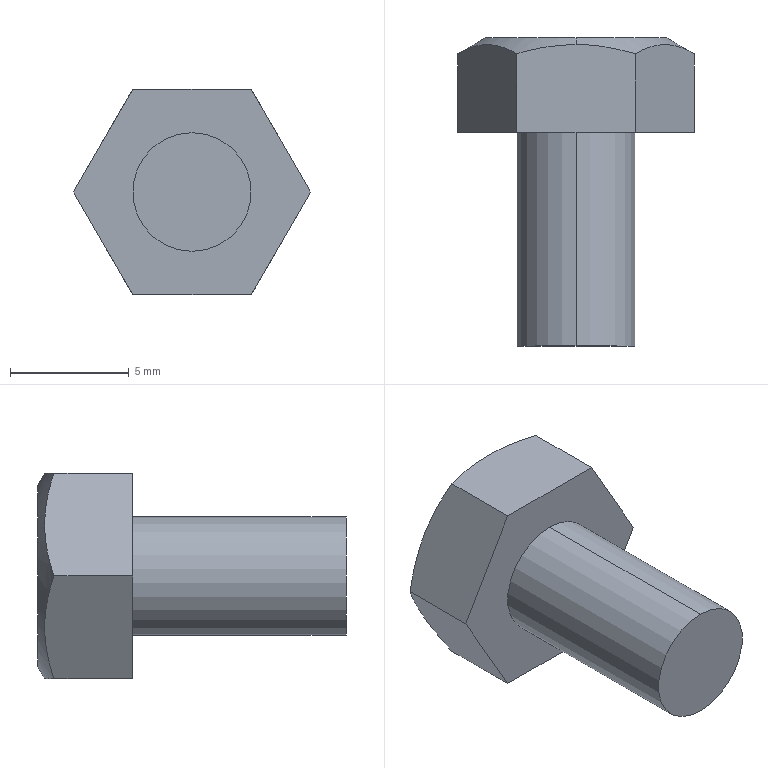Part | SolidWorks | features ICE 2, Extrusion 1 | 1 solid | 13 faces | box 10 x 13 x 8.66 mm | volume 432.272 mm3 | plane 9 | cylinder 2 | cone 2 | commonest cylinder face diameters 5 x2
STEP:
#1=CARTESIAN_POINT('',(0.,-0.3543,-0.09843));
#2=VERTEX_POINT('',#1);
#3=CARTESIAN_POINT('',(0.,-0.3543,0.09843));
#4=VERTEX_POINT('',#3);
#5=CARTESIAN_POINT('',(0.,-0.3543,0.));
#6=DIRECTION('',(0.,-1.,0.));
#7=DIRECTION('',(0.,0.,-1.));
#8=AXIS2_PLACEMENT_3D('',#5,#6,#7);
#9=CIRCLE('',#8,0.09843);
#10=EDGE_CURVE('',#2,#4,#9,.T.);
#11=ORIENTED_EDGE('',*,*,#10,.F.);
#12=CARTESIAN_POINT('',(0.,0.,-0.09843));
#13=VERTEX_POINT('',#12);
#14=CARTESIAN_POINT('',(0.,-0.3543,-0.09843));
#15=DIRECTION('',(0.,1.,0.));
#16=VECTOR('',#15,39.37);
#17=LINE('',#14,#16);
#18=EDGE_CURVE('',#2,#13,#17,.T.);
#19=ORIENTED_EDGE('',*,*,#18,.T.);
#20=CARTESIAN_POINT('',(0.,0.,0.09843));
#21=VERTEX_POINT('',#20);
#22=CARTESIAN_POINT('',(0.,0.,0.));
#23=DIRECTION('',(0.,-1.,0.));
#24=DIRECTION('',(0.,0.,1.));
#25=AXIS2_PLACEMENT_3D('',#22,#23,#24);
#26=CIRCLE('',#25,0.09843);
#27=EDGE_CURVE('',#13,#21,#26,.T.);
#28=ORIENTED_EDGE('',*,*,#27,.T.);
#29=CARTESIAN_POINT('',(0.,-0.3543,0.09843));
#30=DIRECTION('',(0.,1.,0.));
#31=VECTOR('',#30,39.37);
#32=LINE('',#29,#31);
#33=EDGE_CURVE('',#4,#21,#32,.T.);
#34=ORIENTED_EDGE('',*,*,#33,.F.);
#35=EDGE_LOOP('',(#11,#19,#28,#34));
#36=FACE_OUTER_BOUND('',#35,.T.);
#37=CARTESIAN_POINT('',(0.,-0.3543,0.));
#38=DIRECTION('',(0.,1.,0.));
#39=DIRECTION('',(0.,0.,1.));
#40=AXIS2_PLACEMENT_3D('',#37,#38,#39);
#41=CYLINDRICAL_SURFACE('',#40,0.09843);
#42=ADVANCED_FACE('',(#36),#41,.T.);
#43=CARTESIAN_POINT('',(0.,0.1575,-0.1511));
#44=VERTEX_POINT('',#43);
#45=CARTESIAN_POINT('',(0.,0.1575,0.1511));
#46=VERTEX_POINT('',#45);
#47=CARTESIAN_POINT('',(0.,0.1575,0.));
#48=DIRECTION('',(0.,1.,0.));
#49=DIRECTION('',(0.,0.,1.));
#50=AXIS2_PLACEMENT_3D('',#47,#48,#49);
#51=CIRCLE('',#50,0.1511);
#52=EDGE_CURVE('',#44,#46,#51,.T.);
#53=ORIENTED_EDGE('',*,*,#52,.F.);
#54=CARTESIAN_POINT('',(0.,0.1463,-0.1705));
#55=VERTEX_POINT('',#54);
#56=CARTESIAN_POINT('',(0.,0.1575,-0.1511));
#57=DIRECTION('',(0.,-0.5,-0.866));
#58=VECTOR('',#57,39.37);
#59=LINE('',#56,#58);
#60=EDGE_CURVE('',#44,#55,#59,.T.);
#61=ORIENTED_EDGE('',*,*,#60,.T.);
#62=CARTESIAN_POINT('',(-0.09843,0.1311,-0.1705));
#63=VERTEX_POINT('',#62);
#64=CARTESIAN_POINT('',(0.,0.1463,-0.1705));
#65=CARTESIAN_POINT('',(-0.01665,0.1463,-0.1705));
#66=CARTESIAN_POINT('',(-0.03318,0.1449,-0.1705));
#67=CARTESIAN_POINT('',(-0.06601,0.1396,-0.1705));
#68=CARTESIAN_POINT('',(-0.0824,0.1357,-0.1705));
#69=CARTESIAN_POINT('',(-0.09843,0.1311,-0.1705));
#70=B_SPLINE_CURVE_WITH_KNOTS('',3,(#64,#65,#66,#67,#68,#69),.UNSPECIFIED.,.F.,.F.,(4,2,4),(0.01621,0.01748,0.01874),.UNSPECIFIED.);
#71=EDGE_CURVE('',#55,#63,#70,.T.);
#72=ORIENTED_EDGE('',*,*,#71,.T.);
#73=CARTESIAN_POINT('',(-0.1969,0.1311,0.));
#74=VERTEX_POINT('',#73);
#75=CARTESIAN_POINT('',(-0.09843,0.1311,-0.1705));
#76=CARTESIAN_POINT('',(-0.1145,0.1404,-0.1426));
#77=CARTESIAN_POINT('',(-0.1308,0.1463,-0.1144));
#78=CARTESIAN_POINT('',(-0.1559,0.1463,-0.07091));
#79=CARTESIAN_POINT('',(-0.1643,0.1449,-0.05643));
#80=CARTESIAN_POINT('',(-0.1807,0.1396,-0.02799));
#81=CARTESIAN_POINT('',(-0.1888,0.1357,-0.01394));
#82=CARTESIAN_POINT('',(-0.1969,0.1311,0.));
#83=B_SPLINE_CURVE_WITH_KNOTS('',3,(#75,#76,#77,#78,#79,#80,#81,#82),.UNSPECIFIED.,.F.,.F.,(4,2,2,4),(0.000000238,0.002525,0.003788,0.00505),.UNSPECIFIED.);
#84=EDGE_CURVE('',#63,#74,#83,.T.);
#85=ORIENTED_EDGE('',*,*,#84,.T.);
#86=CARTESIAN_POINT('',(-0.09843,0.1311,0.1705));
#87=VERTEX_POINT('',#86);
#88=CARTESIAN_POINT('',(-0.1969,0.1311,0.));
#89=CARTESIAN_POINT('',(-0.1808,0.1404,0.02784));
#90=CARTESIAN_POINT('',(-0.1645,0.1463,0.05609));
#91=CARTESIAN_POINT('',(-0.1394,0.1463,0.09957));
#92=CARTESIAN_POINT('',(-0.131,0.1449,0.114));
#93=CARTESIAN_POINT('',(-0.1146,0.1396,0.1425));
#94=CARTESIAN_POINT('',(-0.1065,0.1357,0.1565));
#95=CARTESIAN_POINT('',(-0.09843,0.1311,0.1705));
#96=B_SPLINE_CURVE_WITH_KNOTS('',3,(#88,#89,#90,#91,#92,#93,#94,#95),.UNSPECIFIED.,.F.,.F.,(4,2,2,4),(0.000000238,0.002525,0.003788,0.00505),.UNSPECIFIED.);
#97=EDGE_CURVE('',#74,#87,#96,.T.);
#98=ORIENTED_EDGE('',*,*,#97,.T.);
#99=CARTESIAN_POINT('',(0.,0.1463,0.1705));
#100=VERTEX_POINT('',#99);
#101=CARTESIAN_POINT('',(-0.09843,0.1311,0.1705));
#102=CARTESIAN_POINT('',(-0.0824,0.1357,0.1705));
#103=CARTESIAN_POINT('',(-0.06601,0.1396,0.1705));
#104=CARTESIAN_POINT('',(-0.03318,0.1449,0.1705));
#105=CARTESIAN_POINT('',(-0.01665,0.1463,0.1705));
#106=CARTESIAN_POINT('',(0.,0.1463,0.1705));
#107=B_SPLINE_CURVE_WITH_KNOTS('',3,(#101,#102,#103,#104,#105,#106),.UNSPECIFIED.,.F.,.F.,(4,2,4),(0.004612,0.005877,0.007142),.UNSPECIFIED.);
#108=EDGE_CURVE('',#87,#100,#107,.T.);
#109=ORIENTED_EDGE('',*,*,#108,.T.);
#110=CARTESIAN_POINT('',(0.,0.1575,0.1511));
#111=DIRECTION('',(0.,-0.5,0.866));
#112=VECTOR('',#111,39.37);
#113=LINE('',#110,#112);
#114=EDGE_CURVE('',#46,#100,#113,.T.);
#115=ORIENTED_EDGE('',*,*,#114,.F.);
#116=EDGE_LOOP('',(#53,#61,#72,#85,#98,#109,#115));
#117=FACE_OUTER_BOUND('',#116,.T.);
#118=CARTESIAN_POINT('',(0.,0.1575,0.));
#119=DIRECTION('',(0.,-1.,0.));
#120=DIRECTION('',(0.,0.,1.));
#121=AXIS2_PLACEMENT_3D('',#118,#119,#120);
#122=CONICAL_SURFACE('',#121,0.1511,1.047);
#123=ADVANCED_FACE('',(#117),#122,.T.);
#124=CARTESIAN_POINT('',(0.09843,0.,0.1705));
#125=VERTEX_POINT('',#124);
#126=CARTESIAN_POINT('',(0.1969,0.,0.));
#127=VERTEX_POINT('',#126);
#128=CARTESIAN_POINT('',(0.09843,0.,0.1705));
#129=DIRECTION('',(0.5,0.,-0.866));
#130=VECTOR('',#129,39.37);
#131=LINE('',#128,#130);
#132=EDGE_CURVE('',#125,#127,#131,.T.);
#133=ORIENTED_EDGE('',*,*,#132,.F.);
#134=CARTESIAN_POINT('',(-0.09843,0.,0.1705));
#135=VERTEX_POINT('',#134);
#136=CARTESIAN_POINT('',(-0.09843,0.,0.1705));
#137=DIRECTION('',(1.,0.,0.));
#138=VECTOR('',#137,39.37);
#139=LINE('',#136,#138);
#140=EDGE_CURVE('',#135,#125,#139,.T.);
#141=ORIENTED_EDGE('',*,*,#140,.F.);
#142=CARTESIAN_POINT('',(-0.1969,0.,0.));
#143=VERTEX_POINT('',#142);
#144=CARTESIAN_POINT('',(-0.1969,0.,0.));
#145=DIRECTION('',(0.5,0.,0.866));
#146=VECTOR('',#145,39.37);
#147=LINE('',#144,#146);
#148=EDGE_CURVE('',#143,#135,#147,.T.);
#149=ORIENTED_EDGE('',*,*,#148,.F.);
#150=CARTESIAN_POINT('',(-0.09843,0.,-0.1705));
#151=VERTEX_POINT('',#150);
#152=CARTESIAN_POINT('',(-0.09843,0.,-0.1705));
#153=DIRECTION('',(-0.5,0.,0.866));
#154=VECTOR('',#153,39.37);
#155=LINE('',#152,#154);
#156=EDGE_CURVE('',#151,#143,#155,.T.);
#157=ORIENTED_EDGE('',*,*,#156,.F.);
#158=CARTESIAN_POINT('',(0.09843,0.,-0.1705));
#159=VERTEX_POINT('',#158);
#160=CARTESIAN_POINT('',(0.09843,0.,-0.1705));
#161=DIRECTION('',(-1.,0.,0.));
#162=VECTOR('',#161,39.37);
#163=LINE('',#160,#162);
#164=EDGE_CURVE('',#159,#151,#163,.T.);
#165=ORIENTED_EDGE('',*,*,#164,.F.);
#166=CARTESIAN_POINT('',(0.1969,0.,0.));
#167=DIRECTION('',(-0.5,0.,-0.866));
#168=VECTOR('',#167,39.37);
#169=LINE('',#166,#168);
#170=EDGE_CURVE('',#127,#159,#169,.T.);
#171=ORIENTED_EDGE('',*,*,#170,.F.);
#172=EDGE_LOOP('',(#133,#141,#149,#157,#165,#171));
#173=FACE_OUTER_BOUND('',#172,.T.);
#174=CARTESIAN_POINT('',(0.,0.,0.));
#175=DIRECTION('',(0.,-1.,0.));
#176=DIRECTION('',(0.,0.,1.));
#177=AXIS2_PLACEMENT_3D('',#174,#175,#176);
#178=CIRCLE('',#177,0.09843);
#179=EDGE_CURVE('',#21,#13,#178,.T.);
#180=ORIENTED_EDGE('',*,*,#179,.F.);
#181=ORIENTED_EDGE('',*,*,#27,.F.);
#182=EDGE_LOOP('',(#180,#181));
#183=FACE_BOUND('',#182,.T.);
#184=CARTESIAN_POINT('',(0.,0.,0.));
#185=DIRECTION('',(0.,1.,0.));
#186=DIRECTION('',(0.,0.,1.));
#187=AXIS2_PLACEMENT_3D('',#184,#185,#186);
#188=PLANE('',#187);
#189=ADVANCED_FACE('',(#173,#183),#188,.F.);
#190=CARTESIAN_POINT('',(0.09843,0.1311,0.1705));
#191=VERTEX_POINT('',#190);
#192=CARTESIAN_POINT('',(0.1969,0.1311,0.));
#193=VERTEX_POINT('',#192);
#194=CARTESIAN_POINT('',(0.09843,0.1311,0.1705));
#195=CARTESIAN_POINT('',(0.1145,0.1404,0.1426));
#196=CARTESIAN_POINT('',(0.1308,0.1463,0.1144));
#197=CARTESIAN_POINT('',(0.1559,0.1463,0.07091));
#198=CARTESIAN_POINT('',(0.1643,0.1449,0.05643));
#199=CARTESIAN_POINT('',(0.1807,0.1396,0.02799));
#200=CARTESIAN_POINT('',(0.1888,0.1357,0.01394));
#201=CARTESIAN_POINT('',(0.1969,0.1311,0.));
#202=B_SPLINE_CURVE_WITH_KNOTS('',3,(#194,#195,#196,#197,#198,#199,#200,#201),.UNSPECIFIED.,.F.,.F.,(4,2,2,4),(0.000000238,0.002525,0.003788,0.00505),.UNSPECIFIED.);
#203=EDGE_CURVE('',#191,#193,#202,.T.);
#204=ORIENTED_EDGE('',*,*,#203,.F.);
#205=CARTESIAN_POINT('',(0.09843,0.1575,0.1705));
#206=DIRECTION('',(0.,-1.,0.));
#207=VECTOR('',#206,39.37);
#208=LINE('',#205,#207);
#209=EDGE_CURVE('',#191,#125,#208,.T.);
#210=ORIENTED_EDGE('',*,*,#209,.T.);
#211=ORIENTED_EDGE('',*,*,#132,.T.);
#212=CARTESIAN_POINT('',(0.1969,0.1575,0.));
#213=DIRECTION('',(0.,-1.,0.));
#214=VECTOR('',#213,39.37);
#215=LINE('',#212,#214);
#216=EDGE_CURVE('',#193,#127,#215,.T.);
#217=ORIENTED_EDGE('',*,*,#216,.F.);
#218=EDGE_LOOP('',(#204,#210,#211,#217));
#219=FACE_OUTER_BOUND('',#218,.T.);
#220=CARTESIAN_POINT('',(0.09843,0.1575,0.1705));
#221=DIRECTION('',(-0.866,0.,-0.5));
#222=DIRECTION('',(-0.5,0.,0.866));
#223=AXIS2_PLACEMENT_3D('',#220,#221,#222);
#224=PLANE('',#223);
#225=ADVANCED_FACE('',(#219),#224,.F.);
#226=CARTESIAN_POINT('',(0.09843,0.1311,-0.1705));
#227=VERTEX_POINT('',#226);
#228=CARTESIAN_POINT('',(0.1969,0.1311,0.));
#229=CARTESIAN_POINT('',(0.1808,0.1404,-0.02784));
#230=CARTESIAN_POINT('',(0.1645,0.1463,-0.05609));
#231=CARTESIAN_POINT('',(0.1394,0.1463,-0.09957));
#232=CARTESIAN_POINT('',(0.131,0.1449,-0.114));
#233=CARTESIAN_POINT('',(0.1146,0.1396,-0.1425));
#234=CARTESIAN_POINT('',(0.1065,0.1357,-0.1565));
#235=CARTESIAN_POINT('',(0.09843,0.1311,-0.1705));
#236=B_SPLINE_CURVE_WITH_KNOTS('',3,(#228,#229,#230,#231,#232,#233,#234,#235),.UNSPECIFIED.,.F.,.F.,(4,2,2,4),(0.000000238,0.002525,0.003788,0.00505),.UNSPECIFIED.);
#237=EDGE_CURVE('',#193,#227,#236,.T.);
#238=ORIENTED_EDGE('',*,*,#237,.F.);
#239=ORIENTED_EDGE('',*,*,#216,.T.);
#240=ORIENTED_EDGE('',*,*,#170,.T.);
#241=CARTESIAN_POINT('',(0.09843,0.1575,-0.1705));
#242=DIRECTION('',(0.,-1.,0.));
#243=VECTOR('',#242,39.37);
#244=LINE('',#241,#243);
#245=EDGE_CURVE('',#227,#159,#244,.T.);
#246=ORIENTED_EDGE('',*,*,#245,.F.);
#247=EDGE_LOOP('',(#238,#239,#240,#246));
#248=FACE_OUTER_BOUND('',#247,.T.);
#249=CARTESIAN_POINT('',(0.1969,0.1575,0.));
#250=DIRECTION('',(-0.866,0.,0.5));
#251=DIRECTION('',(0.5,0.,0.866));
#252=AXIS2_PLACEMENT_3D('',#249,#250,#251);
#253=PLANE('',#252);
#254=ADVANCED_FACE('',(#248),#253,.F.);
#255=CARTESIAN_POINT('',(0.09843,0.1311,-0.1705));
#256=CARTESIAN_POINT('',(0.08251,0.1357,-0.1705));
#257=CARTESIAN_POINT('',(0.06639,0.1395,-0.1705));
#258=CARTESIAN_POINT('',(0.03354,0.1448,-0.1705));
#259=CARTESIAN_POINT('',(0.01666,0.1463,-0.1705));
#260=CARTESIAN_POINT('',(0.,0.1463,-0.1705));
#261=B_SPLINE_CURVE_WITH_KNOTS('',3,(#255,#256,#257,#258,#259,#260),.UNSPECIFIED.,.F.,.F.,(4,2,4),(0.01368,0.01495,0.01621),.UNSPECIFIED.);
#262=EDGE_CURVE('',#227,#55,#261,.T.);
#263=ORIENTED_EDGE('',*,*,#262,.F.);
#264=ORIENTED_EDGE('',*,*,#245,.T.);
#265=ORIENTED_EDGE('',*,*,#164,.T.);
#266=CARTESIAN_POINT('',(-0.09843,0.1575,-0.1705));
#267=DIRECTION('',(0.,-1.,0.));
#268=VECTOR('',#267,39.37);
#269=LINE('',#266,#268);
#270=EDGE_CURVE('',#63,#151,#269,.T.);
#271=ORIENTED_EDGE('',*,*,#270,.F.);
#272=ORIENTED_EDGE('',*,*,#71,.F.);
#273=EDGE_LOOP('',(#263,#264,#265,#271,#272));
#274=FACE_OUTER_BOUND('',#273,.T.);
#275=CARTESIAN_POINT('',(0.09843,0.1575,-0.1705));
#276=DIRECTION('',(0.,0.,1.));
#277=DIRECTION('',(1.,0.,0.));
#278=AXIS2_PLACEMENT_3D('',#275,#276,#277);
#279=PLANE('',#278);
#280=ADVANCED_FACE('',(#274),#279,.F.);
#281=ORIENTED_EDGE('',*,*,#84,.F.);
#282=ORIENTED_EDGE('',*,*,#270,.T.);
#283=ORIENTED_EDGE('',*,*,#156,.T.);
#284=CARTESIAN_POINT('',(-0.1969,0.1575,0.));
#285=DIRECTION('',(0.,-1.,0.));
#286=VECTOR('',#285,39.37);
#287=LINE('',#284,#286);
#288=EDGE_CURVE('',#74,#143,#287,.T.);
#289=ORIENTED_EDGE('',*,*,#288,.F.);
#290=EDGE_LOOP('',(#281,#282,#283,#289));
#291=FACE_OUTER_BOUND('',#290,.T.);
#292=CARTESIAN_POINT('',(-0.09843,0.1575,-0.1705));
#293=DIRECTION('',(0.866,0.,0.5));
#294=DIRECTION('',(0.5,0.,-0.866));
#295=AXIS2_PLACEMENT_3D('',#292,#293,#294);
#296=PLANE('',#295);
#297=ADVANCED_FACE('',(#291),#296,.F.);
#298=ORIENTED_EDGE('',*,*,#97,.F.);
#299=ORIENTED_EDGE('',*,*,#288,.T.);
#300=ORIENTED_EDGE('',*,*,#148,.T.);
#301=CARTESIAN_POINT('',(-0.09843,0.1575,0.1705));
#302=DIRECTION('',(0.,-1.,0.));
#303=VECTOR('',#302,39.37);
#304=LINE('',#301,#303);
#305=EDGE_CURVE('',#87,#135,#304,.T.);
#306=ORIENTED_EDGE('',*,*,#305,.F.);
#307=EDGE_LOOP('',(#298,#299,#300,#306));
#308=FACE_OUTER_BOUND('',#307,.T.);
#309=CARTESIAN_POINT('',(-0.1969,0.1575,0.));
#310=DIRECTION('',(0.866,0.,-0.5));
#311=DIRECTION('',(-0.5,0.,-0.866));
#312=AXIS2_PLACEMENT_3D('',#309,#310,#311);
#313=PLANE('',#312);
#314=ADVANCED_FACE('',(#308),#313,.F.);
#315=ORIENTED_EDGE('',*,*,#108,.F.);
#316=ORIENTED_EDGE('',*,*,#305,.T.);
#317=ORIENTED_EDGE('',*,*,#140,.T.);
#318=ORIENTED_EDGE('',*,*,#209,.F.);
#319=CARTESIAN_POINT('',(0.,0.1463,0.1705));
#320=CARTESIAN_POINT('',(0.01666,0.1463,0.1705));
#321=CARTESIAN_POINT('',(0.03354,0.1448,0.1705));
#322=CARTESIAN_POINT('',(0.06639,0.1395,0.1705));
#323=CARTESIAN_POINT('',(0.08251,0.1357,0.1705));
#324=CARTESIAN_POINT('',(0.09843,0.1311,0.1705));
#325=B_SPLINE_CURVE_WITH_KNOTS('',3,(#319,#320,#321,#322,#323,#324),.UNSPECIFIED.,.F.,.F.,(4,2,4),(0.007142,0.008409,0.009675),.UNSPECIFIED.);
#326=EDGE_CURVE('',#100,#191,#325,.T.);
#327=ORIENTED_EDGE('',*,*,#326,.F.);
#328=EDGE_LOOP('',(#315,#316,#317,#318,#327));
#329=FACE_OUTER_BOUND('',#328,.T.);
#330=CARTESIAN_POINT('',(-0.09843,0.1575,0.1705));
#331=DIRECTION('',(0.,0.,-1.));
#332=DIRECTION('',(-1.,0.,0.));
#333=AXIS2_PLACEMENT_3D('',#330,#331,#332);
#334=PLANE('',#333);
#335=ADVANCED_FACE('',(#329),#334,.F.);
#336=ORIENTED_EDGE('',*,*,#60,.F.);
#337=CARTESIAN_POINT('',(0.,0.1575,0.));
#338=DIRECTION('',(0.,1.,0.));
#339=DIRECTION('',(0.,0.,1.));
#340=AXIS2_PLACEMENT_3D('',#337,#338,#339);
#341=CIRCLE('',#340,0.1511);
#342=EDGE_CURVE('',#46,#44,#341,.T.);
#343=ORIENTED_EDGE('',*,*,#342,.F.);
#344=ORIENTED_EDGE('',*,*,#114,.T.);
#345=ORIENTED_EDGE('',*,*,#326,.T.);
#346=ORIENTED_EDGE('',*,*,#203,.T.);
#347=ORIENTED_EDGE('',*,*,#237,.T.);
#348=ORIENTED_EDGE('',*,*,#262,.T.);
#349=EDGE_LOOP('',(#336,#343,#344,#345,#346,#347,#348));
#350=FACE_OUTER_BOUND('',#349,.T.);
#351=CARTESIAN_POINT('',(0.,0.1575,0.));
#352=DIRECTION('',(0.,-1.,0.));
#353=DIRECTION('',(0.,0.,1.));
#354=AXIS2_PLACEMENT_3D('',#351,#352,#353);
#355=CONICAL_SURFACE('',#354,0.1511,1.047);
#356=ADVANCED_FACE('',(#350),#355,.T.);
#357=ORIENTED_EDGE('',*,*,#342,.T.);
#358=ORIENTED_EDGE('',*,*,#52,.T.);
#359=EDGE_LOOP('',(#357,#358));
#360=FACE_OUTER_BOUND('',#359,.T.);
#361=CARTESIAN_POINT('',(0.,0.1575,0.));
#362=DIRECTION('',(0.,1.,0.));
#363=DIRECTION('',(0.,0.,1.));
#364=AXIS2_PLACEMENT_3D('',#361,#362,#363);
#365=PLANE('',#364);
#366=ADVANCED_FACE('',(#360),#365,.T.);
#367=ORIENTED_EDGE('',*,*,#18,.F.);
#368=CARTESIAN_POINT('',(0.,-0.3543,0.));
#369=DIRECTION('',(0.,-1.,0.));
#370=DIRECTION('',(0.,0.,-1.));
#371=AXIS2_PLACEMENT_3D('',#368,#369,#370);
#372=CIRCLE('',#371,0.09843);
#373=EDGE_CURVE('',#4,#2,#372,.T.);
#374=ORIENTED_EDGE('',*,*,#373,.F.);
#375=ORIENTED_EDGE('',*,*,#33,.T.);
#376=ORIENTED_EDGE('',*,*,#179,.T.);
#377=EDGE_LOOP('',(#367,#374,#375,#376));
#378=FACE_OUTER_BOUND('',#377,.T.);
#379=CARTESIAN_POINT('',(0.,-0.3543,0.));
#380=DIRECTION('',(0.,1.,0.));
#381=DIRECTION('',(0.,0.,1.));
#382=AXIS2_PLACEMENT_3D('',#379,#380,#381);
#383=CYLINDRICAL_SURFACE('',#382,0.09843);
#384=ADVANCED_FACE('',(#378),#383,.T.);
#385=ORIENTED_EDGE('',*,*,#373,.T.);
#386=ORIENTED_EDGE('',*,*,#10,.T.);
#387=EDGE_LOOP('',(#385,#386));
#388=FACE_OUTER_BOUND('',#387,.T.);
#389=CARTESIAN_POINT('',(0.,-0.3543,0.));
#390=DIRECTION('',(0.,-1.,0.));
#391=DIRECTION('',(0.,0.,-1.));
#392=AXIS2_PLACEMENT_3D('',#389,#390,#391);
#393=PLANE('',#392);
#394=ADVANCED_FACE('',(#388),#393,.T.);
#395=CLOSED_SHELL('',(#42,#123,#189,#225,#254,#280,#297,#314,#335,#356,#366,#384,#394));
#396=MANIFOLD_SOLID_BREP('',#395);
#397=CARTESIAN_POINT('',(0.,0.,0.));
#398=DIRECTION('',(0.,0.,1.));
#399=DIRECTION('',(1.,0.,0.));
#400=AXIS2_PLACEMENT_3D('',#397,#398,#399);
#401=(LENGTH_UNIT()NAMED_UNIT(*)SI_UNIT($,.METRE.));
#402=LENGTH_MEASURE_WITH_UNIT(LENGTH_MEASURE(0.0254),#401);
#403=DIMENSIONAL_EXPONENTS(1.,0.,0.,0.,0.,0.,0.);
#404=(CONVERSION_BASED_UNIT('INCH',#402)LENGTH_UNIT()NAMED_UNIT(#403));
#405=UNCERTAINTY_MEASURE_WITH_UNIT(LENGTH_MEASURE(0.00001),#404,'','');
#406=(NAMED_UNIT(*)PLANE_ANGLE_UNIT()SI_UNIT($,.RADIAN.));
#407=(NAMED_UNIT(*)SI_UNIT($,.STERADIAN.)SOLID_ANGLE_UNIT());
#408=(GEOMETRIC_REPRESENTATION_CONTEXT(3)GLOBAL_UNCERTAINTY_ASSIGNED_CONTEXT((#405))GLOBAL_UNIT_ASSIGNED_CONTEXT((#404,#406,#407))REPRESENTATION_CONTEXT('',''));
#409=ADVANCED_BREP_SHAPE_REPRESENTATION('',(#396,#400),#408);